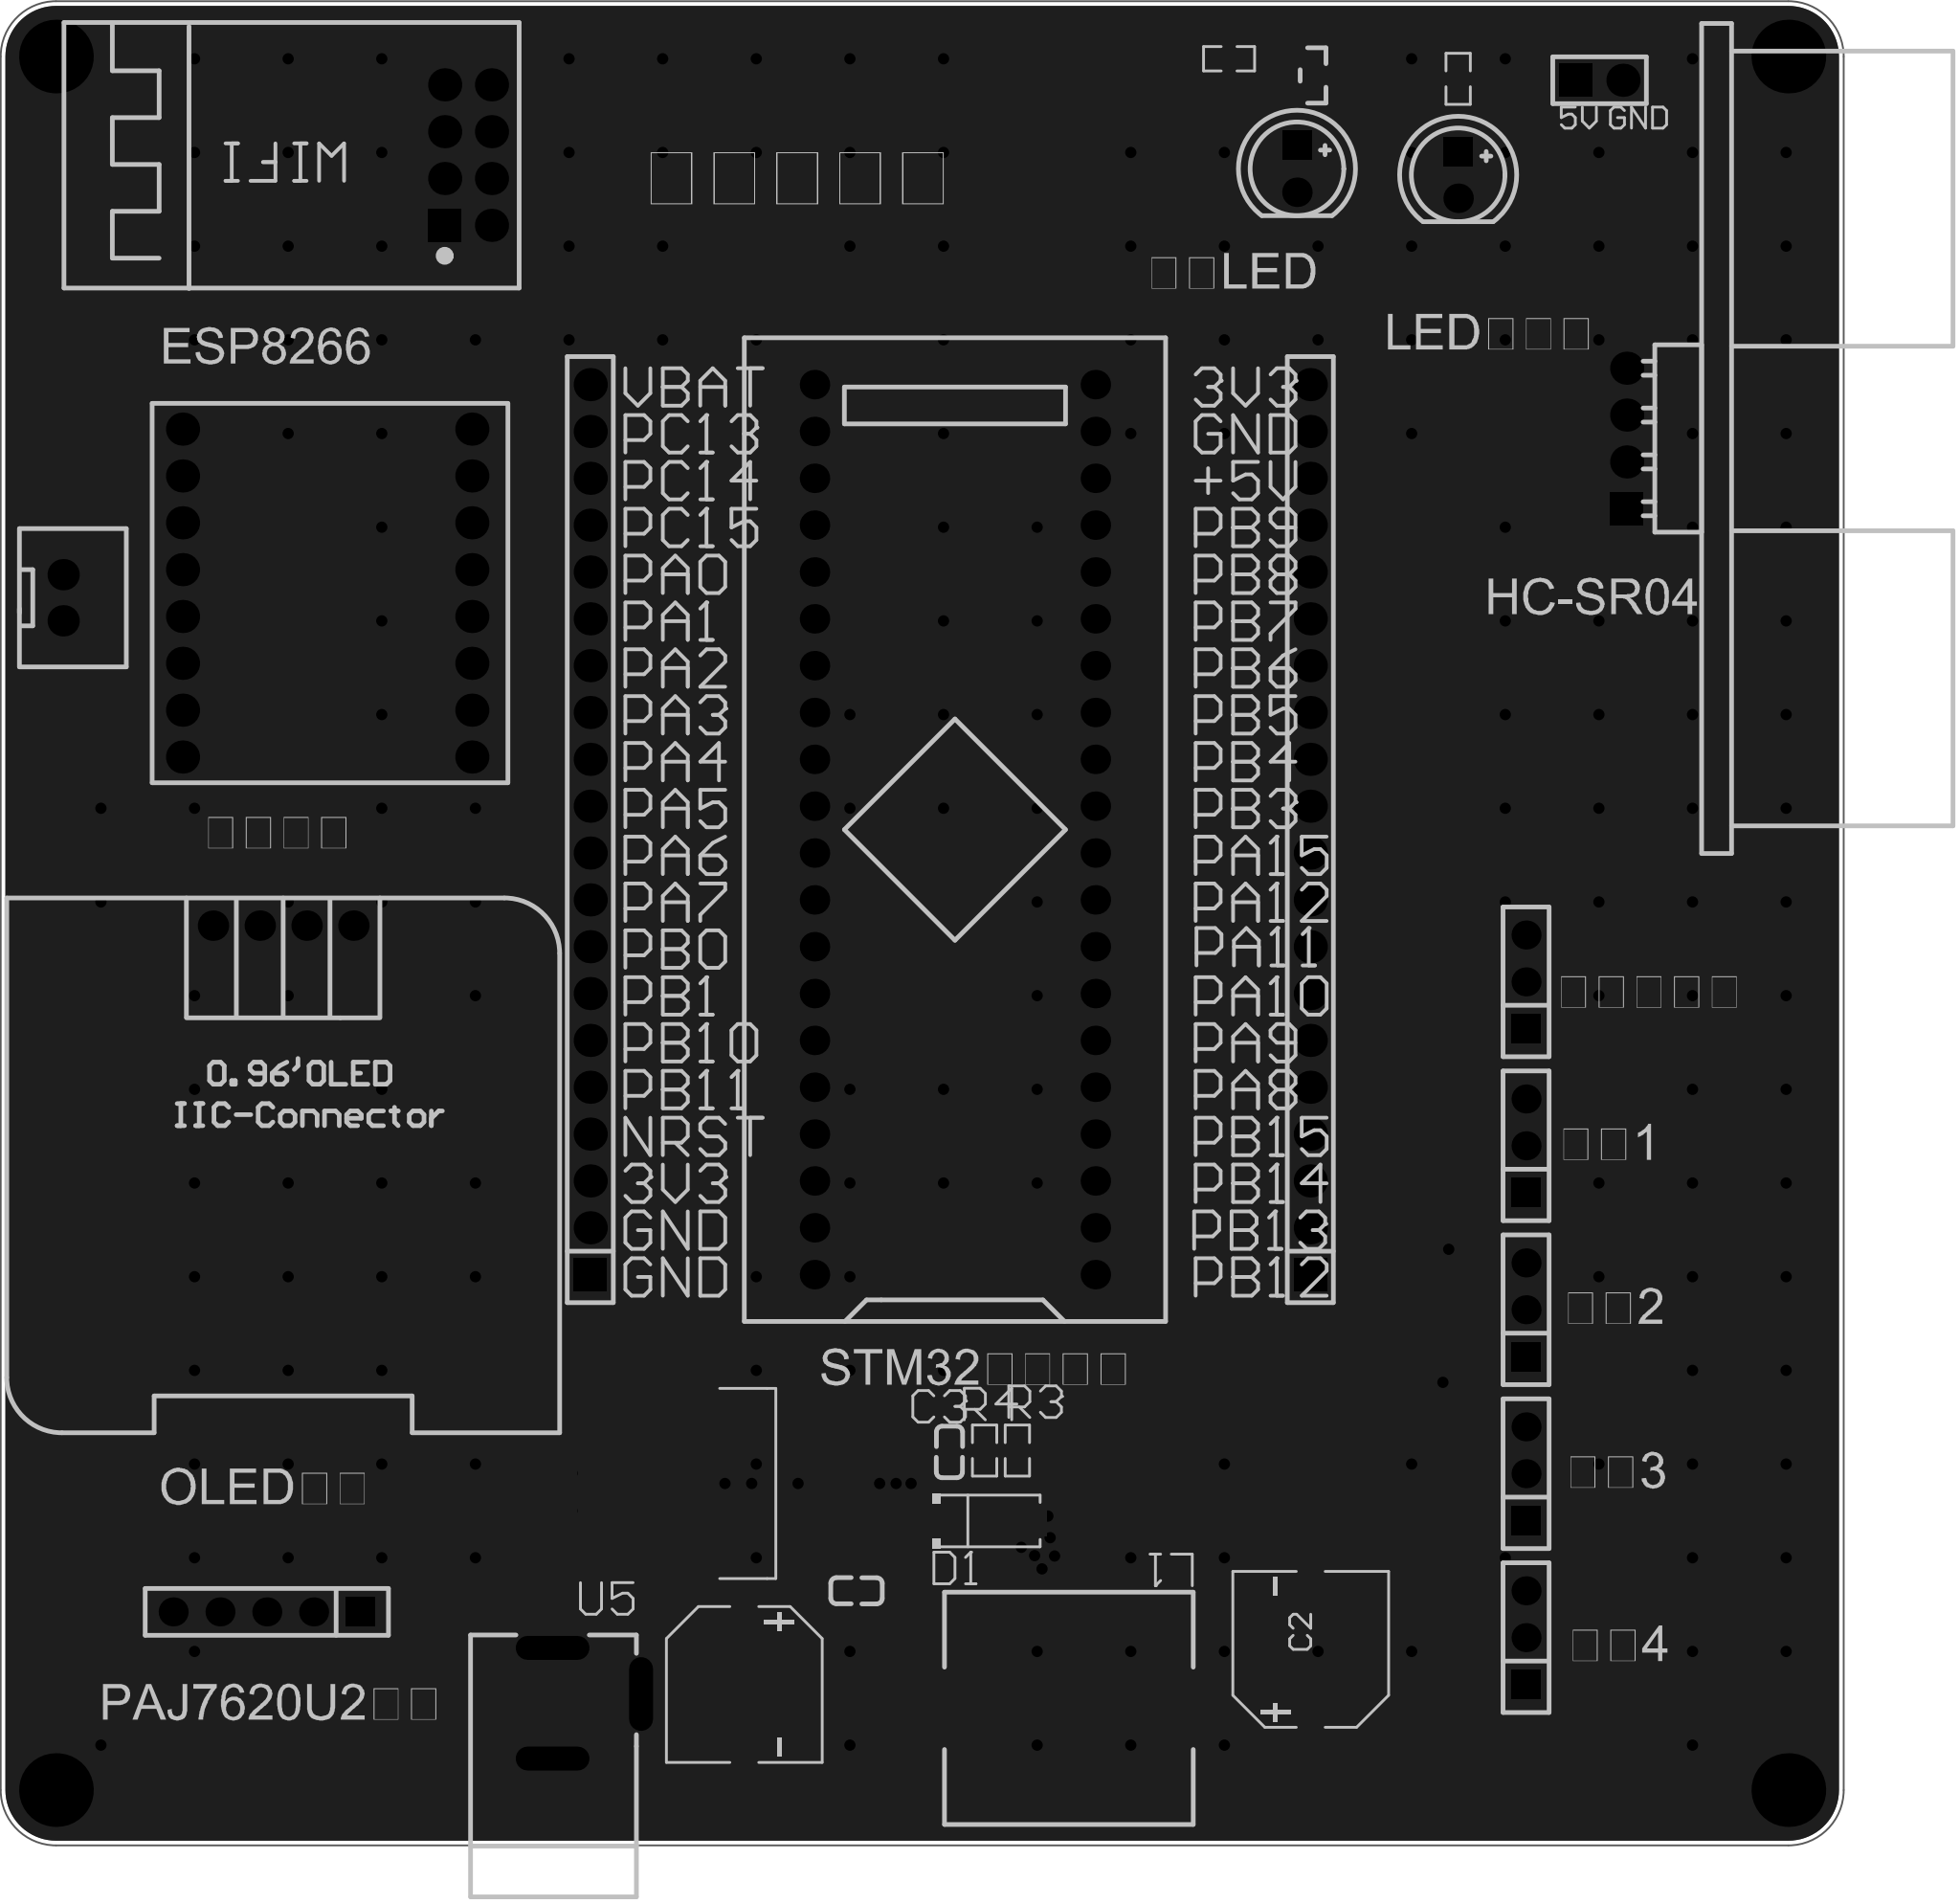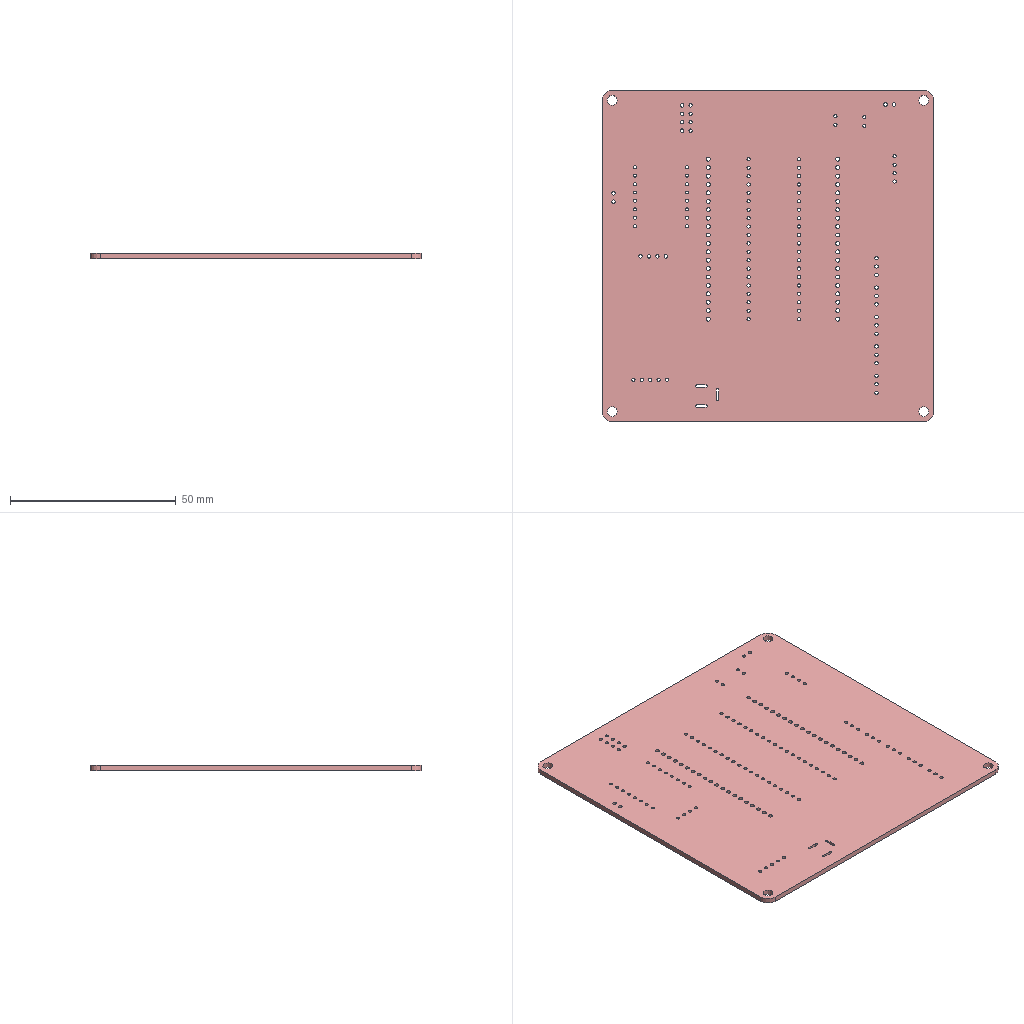Circuit board layout | Altium Designer | box 100 x 100 x 1.6 mm
Layer stack:
# Altium Designer layer stack of  (unit mm; dielectric type: 0 none, 1 core, 2 prepreg, 3 surface material)
index,name,kind,layer,copper_thickness_mm,dielectric_type,dielectric_thickness_mm,dielectric_material,dielectric_constant
0,Top Paste Mask Layer,other,,,,,,
1,Top Silkscreen Layer,other,,,,,,
2,Top Solder Mask Layer,dielectric,,,3,0.01,,3.3
3,Top Layer,copper,Top Layer,0.035,,,,
4,Dielectric1,dielectric,,,3,1.51,FR4,4.5
5,Bottom Layer,copper,Bottom Layer,0.035,,,,
6,Bottom Solder Mask Layer,dielectric,,,3,0.01,,3.3
7,Bottom Silkscreen Layer,other,,,,,,
8,Bottom Paste Mask Layer,other,,,,,,
# drill layer pairs: low layer,high layer
drill_pair,Top Layer,Bottom Layer
Part placement:
Designator,Comment,Layer,Footprint,Center-X(mm),Center-Y(mm),Rotation
U1,STM32F103C8T6-Card,TopLayer,CONN-TH_L53.3-W22.9_STM32F103C8T6-CARD,132.334,134.112,90
H1,,TopLayer,HDR-TH_20P-P2.54-V-F,151.617,134.112,90
H2,,TopLayer,HDR-TH_20P-P2.54-V-F,112.546,134.112,90
H3,,TopLayer,HDR-TH_3P-P2.54-V-F,163.322,108.077,90
H4,,TopLayer,HDR-TH_3P-P2.54-V-F,163.322,116.967,90
H5,,TopLayer,HDR-TH_3P-P2.54-V-F,163.322,99.187,90
OLED1,,TopLayer,0.96OLED_4P,95.885,128.905,0
R1,300,TopLayer,R0603,159.637,174.823,90
U2,Ai-Thinker ESP-01S ESP8266,TopLayer,WIFIM-TH_8P-L24.7-W14.4-P2.54,105.918,170.688,180
U3,HC-SR04,TopLayer,TH_HC-SR04V,168.783,155.321,90
H7,,TopLayer,HDR-TH_3P-P2.54-V-F,163.322,125.857,90
H8,,TopLayer,HDR-TH_3P-P2.54-V-F,163.322,90.297,90
LED1,,TopLayer,LED-TH_5mm,159.637,169.616,270
H6,,TopLayer,HDR-TH_5P-P2.54-V-F,94.996,91.694,180
CN2,XH2.54*2P_直插,TopLayer,CONN-TH_2P-P2.50-XH2.54-2P,83.947,146.685,90
LED3,,TopLayer,LED-TH_5mm,150.89,169.942,270
Q1,,TopLayer,S8050_SOT-23,151.765,175.006,180
R2,20K,TopLayer,R0603,147.207,175.911,0
U4,,TopLayer,tb6612,98.273,146.939,0
L1,,TopLayer,IND-SMD_L13.5-W12.6,138.514,86.465,180
D1,,TopLayer,SMA_L4.4-W2.6-LS5.0-RD,134.229,96.625,0
R3,,TopLayer,R0603,135.72,100.443,270
R4,,TopLayer,R0603,133.942,100.443,90
C3,,TopLayer,C0603,132.037,100.374,90
U5,,TopLayer,TO-263-5_L10.2-W8.9-P1.70-BR,120.964,98.657,0
DC1,,TopLayer,DC-2.0,112.903,86.741,270
C1,,TopLayer,CAP-SMD_BD8.0-L8.3-W8.3-LS9.0-FD,120.904,87.757,270
C2,,TopLayer,CAP-SMD_BD8.0-L8.3-W8.3-LS9.0-FD,151.638,89.662,90
C4,,TopLayer,C0603,127,92.837,0
H9,,TopLayer,HDR-TH_2P-P2.54-V-M-1,167.31,174.746,0
Pad and via stacks:
# Altium Designer via and pad stacks of  (unit mm). Each distinct definition once, with the count of objects using it.
# via: kind,start_layer,end_layer,hole_mm,diameter_mm,mode(0 simple;1 top-mid-bottom;2 full stack),diameter_per_layer,count,example_net
# pad: kind,layer,hole_mm,hole_type(0 round;1 square;2 slot),plating,top_size,top_shape(1 round;2 rect;3 octagon;9 rounded rect),mid_size,bottom_size,mode,footprint,size_per_layer,count,example
pad,Multi-Layer,3,0,plated,4x4,1,4x4,4x4,0,,,4,1
pad,Multi-Layer,1,0,plated,1.6x1.6,1,1.6x1.6,1.6x1.6,0,CONN-TH_L53.3-W22.9_STM32F103C8T6-CARD,,40,U1.1
pad,Multi-Layer,1.2,0,plated,1.8x1.8,2,1.8x1.8,1.8x1.8,0,HDR-TH_20P-P2.54-V-F,,2,H1.1
pad,Multi-Layer,1.2,0,plated,1.8x1.8,1,1.8x1.8,1.8x1.8,0,HDR-TH_20P-P2.54-V-F,,38,H1.2
pad,Multi-Layer,1.02,0,plated,1.575x1.575,1,1.575x1.575,1.575x1.575,0,HDR-TH_3P-P2.54-V-F,,10,H3.3
pad,Multi-Layer,1.02,0,plated,1.575x1.575,2,1.575x1.575,1.575x1.575,0,HDR-TH_3P-P2.54-V-F,,5,H3.1
pad,Multi-Layer,1,0,plated,1.65x1.65,1,1.65x1.65,1.65x1.65,0,0.96OLED_4P,,4,OLED1.4
pad,Multi-Layer,1,0,plated,1.8x1.8,1,1.8x1.8,1.8x1.8,0,WIFIM-TH_8P-L24.7-W14.4-P2.54,,7,U2.8
pad,Multi-Layer,1,0,plated,1.8x1.8,2,1.8x1.8,1.8x1.8,0,WIFIM-TH_8P-L24.7-W14.4-P2.54,,1,U2.1
pad,Multi-Layer,1.001,0,plated,1.8x1.8,1,1.8x1.8,1.8x1.8,0,TH_HC-SR04V,,3,U3.4
pad,Multi-Layer,1.001,0,plated,1.8x1.8,2,1.8x1.8,1.8x1.8,0,TH_HC-SR04V,,1,U3.1
pad,Multi-Layer,1,0,plated,1.6x1.6,2,1.6x1.6,1.6x1.6,0,LED-TH_5mm,,2,LED1.1
pad,Multi-Layer,1,0,plated,1.6x1.6,1,1.6x1.6,1.6x1.6,0,LED-TH_5mm,,2,LED1.2
pad,Multi-Layer,1.02,0,plated,1.575x1.575,1,1.575x1.575,1.575x1.575,0,HDR-TH_5P-P2.54-V-F,,4,H6.5
pad,Multi-Layer,1.02,0,plated,1.575x1.575,2,1.575x1.575,1.575x1.575,0,HDR-TH_5P-P2.54-V-F,,1,H6.1
pad,Multi-Layer,1.05,0,plated,1.7x1.7,1,1.7x1.7,1.7x1.7,0,CONN-TH_2P-P2.50-XH2.54-2P,,2,CN2.2
pad,Multi-Layer,0.9,0,plated,1.8x1.8,1,1.8x1.8,1.8x1.8,0,tb6612,,16,U4.1
pad,Multi-Layer,0.8001,2,plated,4x1.3,1,4x1.3,4x1.3,0,DC-2.0,,3,DC1.2
pad,Multi-Layer,1.1,0,plated,1.8x1.8,1,1.8x1.8,1.8x1.8,0,HDR-TH_2P-P2.54-V-M-1,,1,H9.2
pad,Multi-Layer,1.1,0,plated,1.8x1.8,2,1.8x1.8,1.8x1.8,0,HDR-TH_2P-P2.54-V-M-1,,1,H9.1
pad,Top Layer,0,0,plated,0.8065x0.864,2,0.8065x0.864,0.8065x0.864,0,R0603,,4,R1.2
pad,Top Layer,0,0,plated,1x0.8,2,1x0.8,1x0.8,0,S8050_SOT-23,,3,Q1.2
pad,Top Layer,0,0,plated,4x3.5,2,4x3.5,4x3.5,0,IND-SMD_L13.5-W12.6,,2,L1.1
pad,Top Layer,0,0,plated,1.801x1.699,2,1.801x1.699,1.801x1.699,0,SMA_L4.4-W2.6-LS5.0-RD,,2,D1.2
pad,Top Layer,0,0,plated,0.8077x0.8636,2,0.8077x0.8636,0.8077x0.8636,0,R0603,,4,R3.2
pad,Top Layer,0,0,plated,0.8001x0.8992,2,0.8001x0.8992,0.8001x0.8992,0,C0603,,4,C3.2
pad,Top Layer,0,0,plated,3.084x1.021,2,3.084x1.021,3.084x1.021,0,TO-263-5_L10.2-W8.9-P1.70-BR,,5,U5.1
pad,Top Layer,0,0,plated,7.521x10.566,2,7.521x10.566,7.521x10.566,0,TO-263-5_L10.2-W8.9-P1.70-BR,,1,U5.6
pad,Top Layer,0,0,plated,3.609x1.26,2,3.609x1.26,3.609x1.26,0,CAP-SMD_BD8.0-L8.3-W8.3-LS9.0-FD,,4,C1.2
via,Top Layer,Bottom Layer,0.3048,0.61,0,,216,GND
Copper pours:
name,layer,net,type(0 solid;1 hatched;2 none)
Bottom Layer-GND,Bottom Layer,GND,0
Top Layer-GND,Top Layer,GND,0